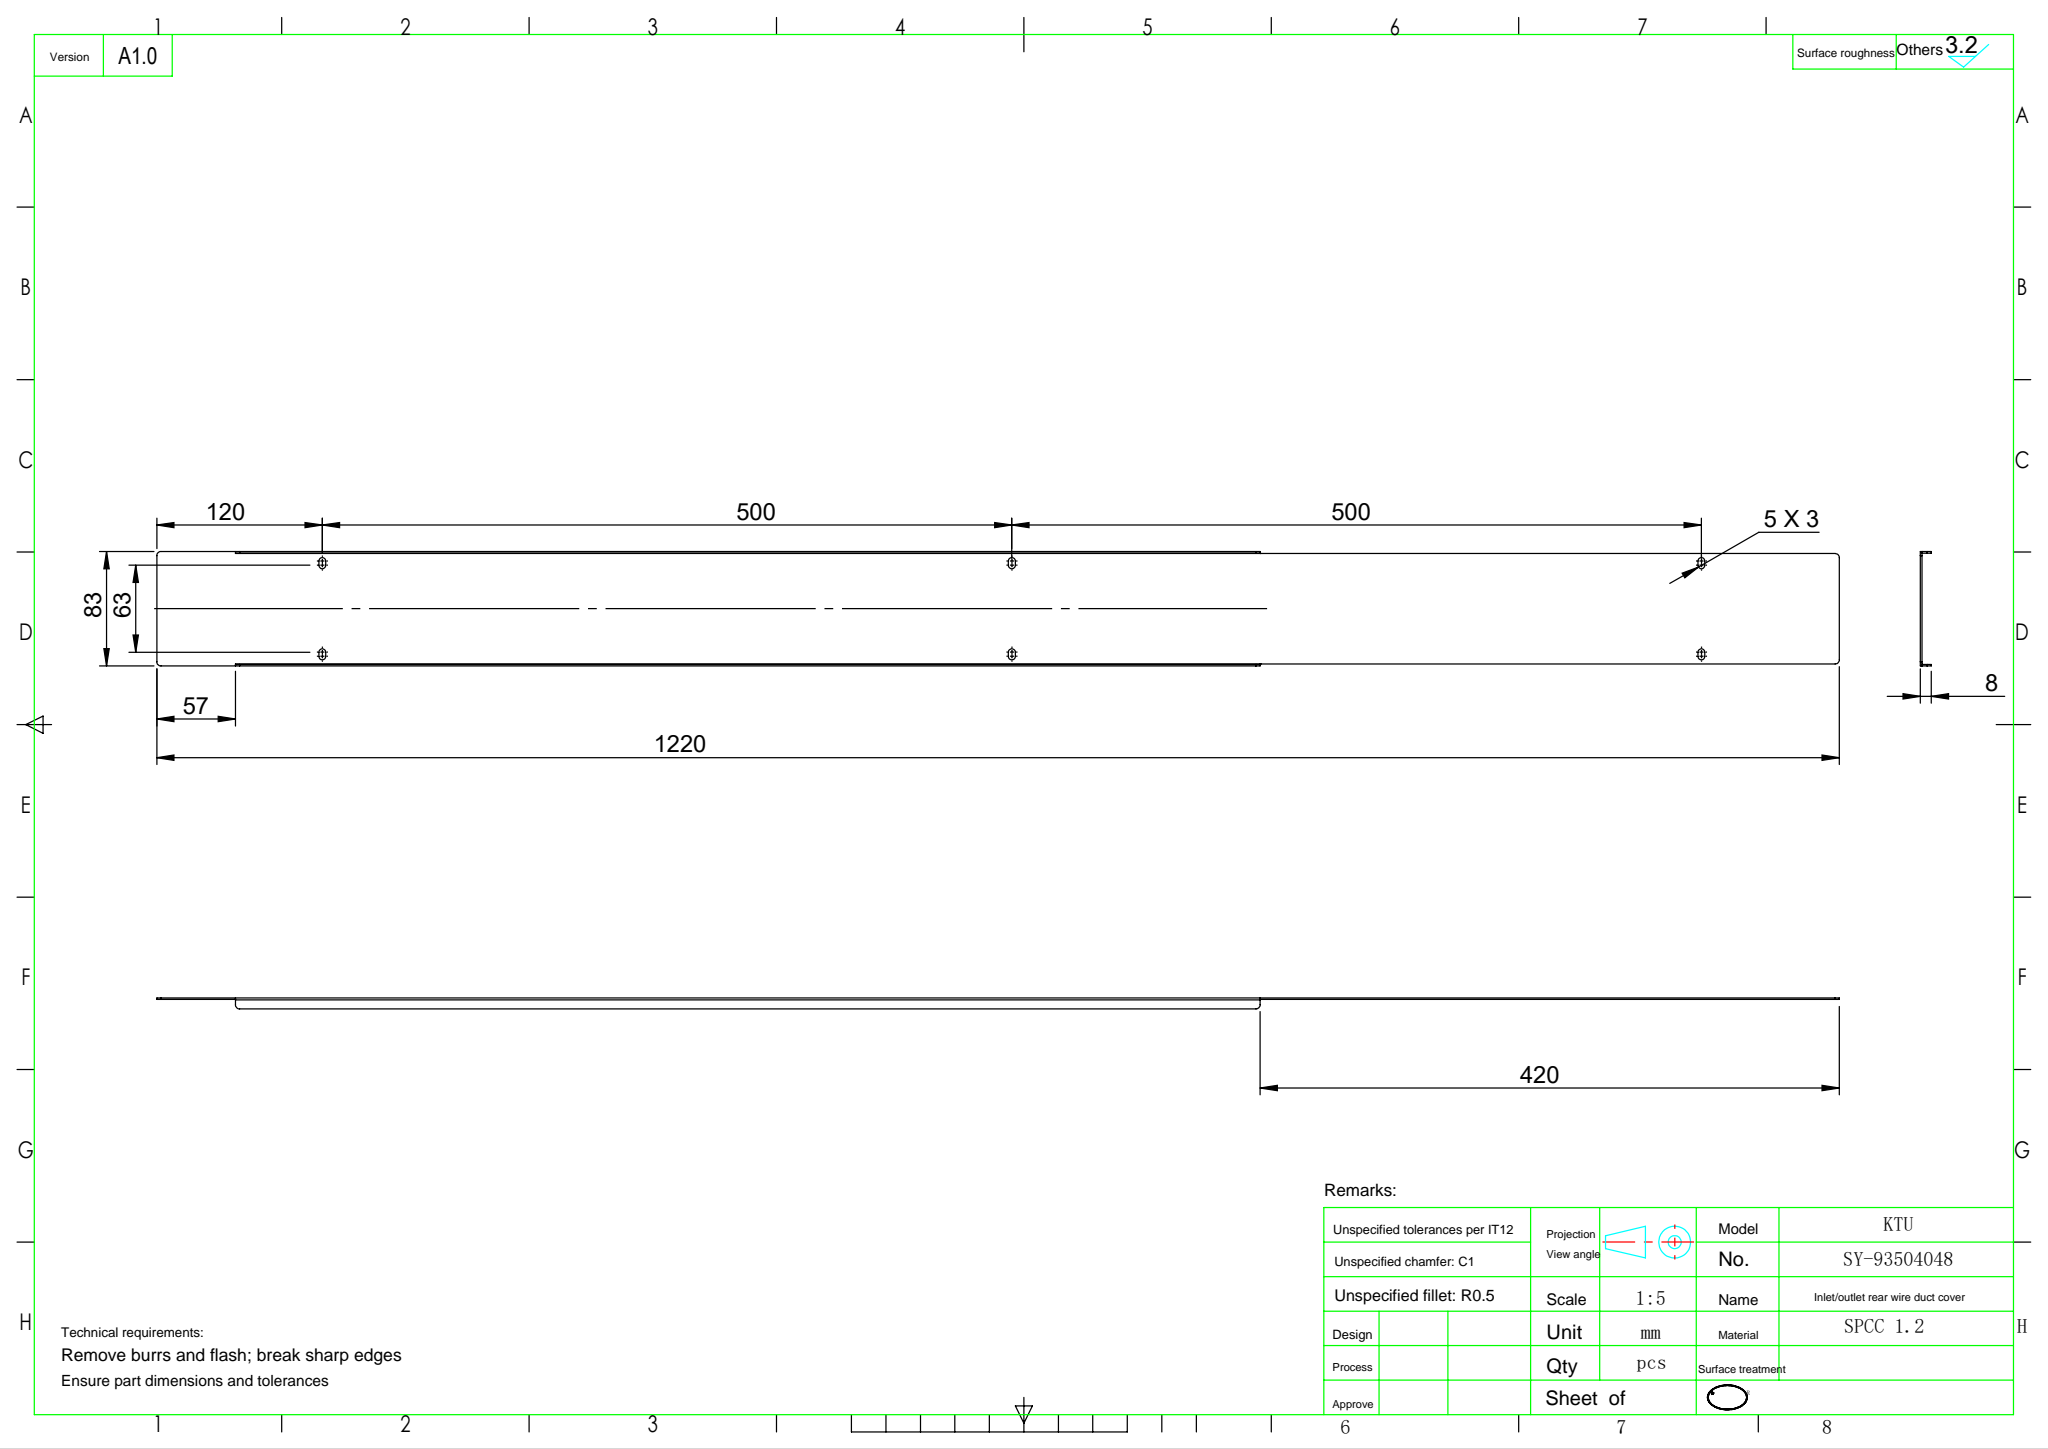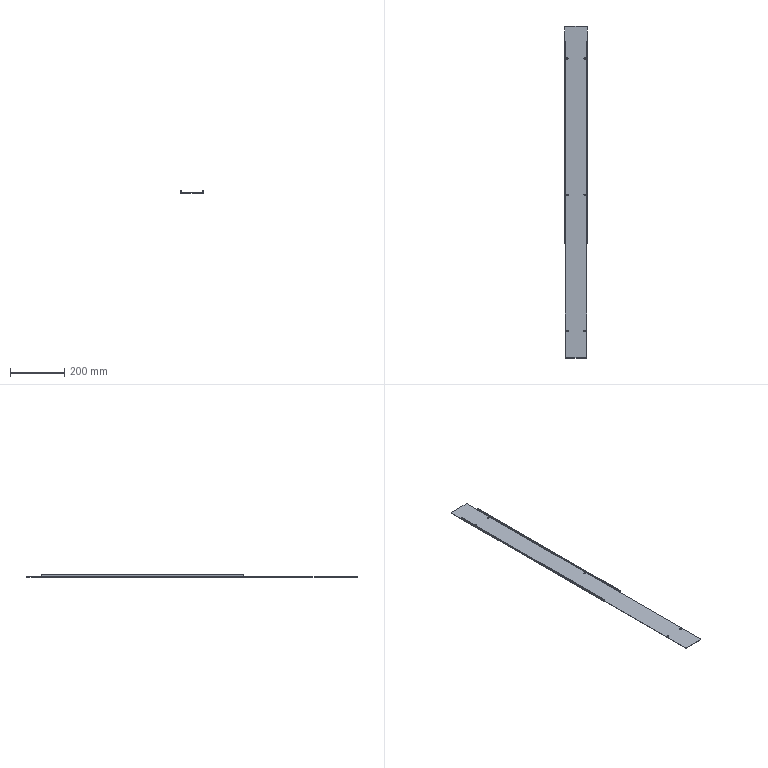Part | SolidWorks | features Fillet 2, ICE 2, EdgeFlange 1, FlatPattern 1, LPattern 1, MoveFace 1, SMBaseFlange 1, SheetMetal 1 | 1 solid | 68 faces | box 83 x 1220 x 8 mm | volume 131246 mm3 | plane 38 | cylinder 30 | commonest cylinder face diameters 5 x18 6 x8 0.4 x2 2.8 x2